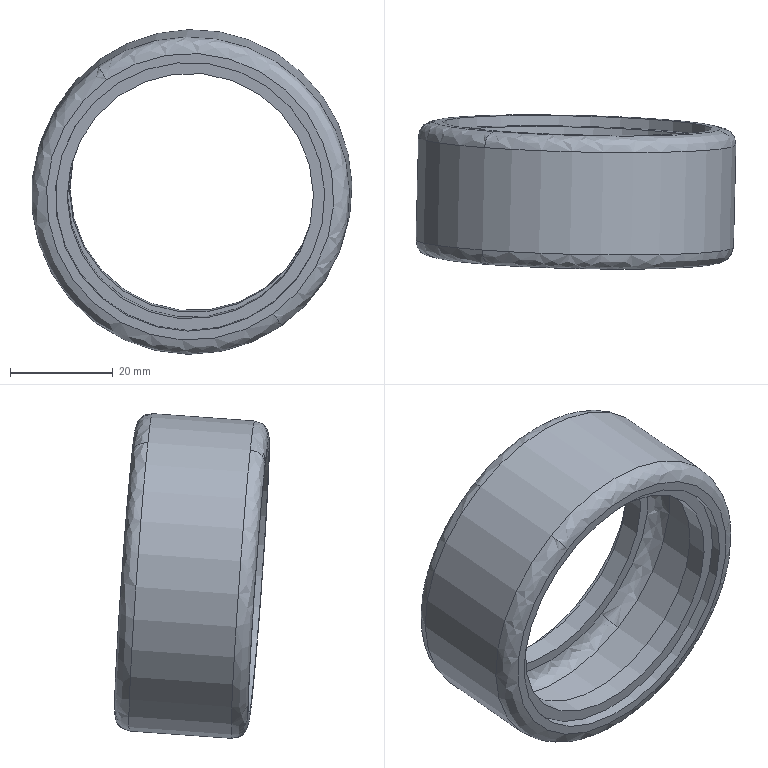Part | STEP file | PNEU | 1 solid | 20 faces | box 62.467 x 30.182 x 63.29 mm | volume 18321 mm3 | spline 8 | cylinder 6 | plane 6 | commonest cylinder face diameters 48 x2 52.5 x2 58 x1 62 x1